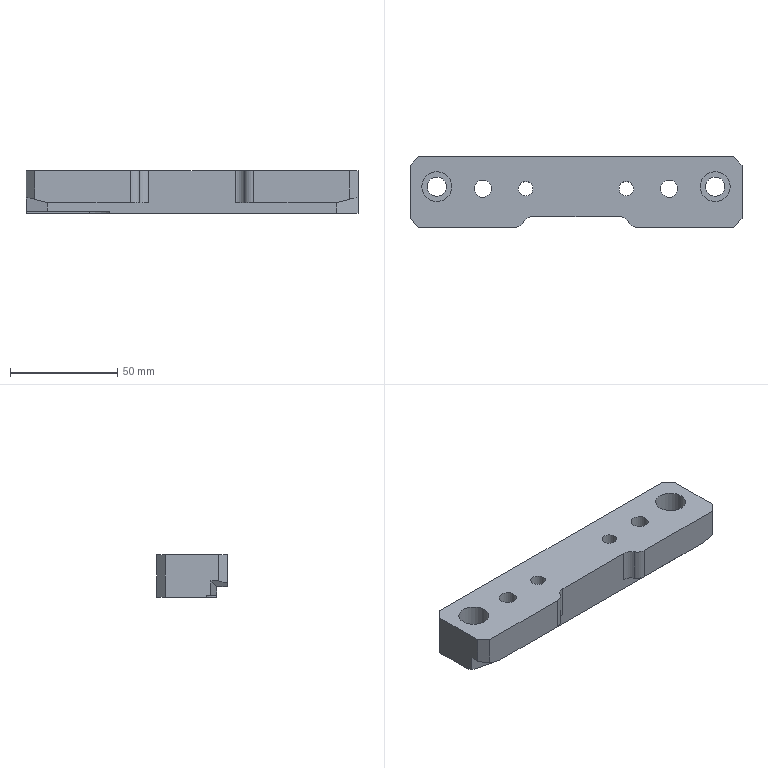Part | NX | features 20 2 | 1 solid | 35 faces | box 155 x 33 x 20 mm | volume 85943 mm3 | plane 22 | cylinder 13 | commonest cylinder face diameters 10 x4 6.8 x2 8.001 x2 9 x2 14 x2 24 x1
STEP:
#1=CARTESIAN_POINT('',(603.057,427.372,-2.5));
#2=VERTEX_POINT('',#1);
#3=CARTESIAN_POINT('',(612.711,422.5,-2.5));
#4=VERTEX_POINT('',#3);
#5=CARTESIAN_POINT('',(603.057,415.372,-2.5));
#6=DIRECTION('',(0.,0.,-1.));
#7=DIRECTION('',(1.,0.,0.));
#8=AXIS2_PLACEMENT_3D('',#5,#6,#7);
#9=CIRCLE('',#8,12.);
#10=EDGE_CURVE('',#2,#4,#9,.T.);
#11=ORIENTED_EDGE('',*,*,#10,.F.);
#12=CARTESIAN_POINT('',(603.057,427.372,-3.5));
#13=VERTEX_POINT('',#12);
#14=CARTESIAN_POINT('',(603.057,427.372,-33.5));
#15=DIRECTION('',(0.,0.,-1.));
#16=VECTOR('',#15,1000.);
#17=LINE('',#14,#16);
#18=EDGE_CURVE('',#2,#13,#17,.T.);
#19=ORIENTED_EDGE('',*,*,#18,.T.);
#20=CARTESIAN_POINT('',(612.711,422.5,-3.5));
#21=VERTEX_POINT('',#20);
#22=CARTESIAN_POINT('',(603.057,415.372,-3.5));
#23=DIRECTION('',(0.,0.,1.));
#24=DIRECTION('',(1.,0.,0.));
#25=AXIS2_PLACEMENT_3D('',#22,#23,#24);
#26=CIRCLE('',#25,12.);
#27=EDGE_CURVE('',#21,#13,#26,.T.);
#28=ORIENTED_EDGE('',*,*,#27,.F.);
#29=CARTESIAN_POINT('',(612.711,422.5,-33.5));
#30=DIRECTION('',(0.,0.,1.));
#31=VECTOR('',#30,1000.);
#32=LINE('',#29,#31);
#33=EDGE_CURVE('',#21,#4,#32,.T.);
#34=ORIENTED_EDGE('',*,*,#33,.T.);
#35=EDGE_LOOP('',(#11,#19,#28,#34));
#36=FACE_BOUND('',#35,.T.);
#37=CARTESIAN_POINT('',(603.057,415.372,-33.5));
#38=DIRECTION('',(0.,0.,1.));
#39=DIRECTION('',(-1.,0.,0.));
#40=AXIS2_PLACEMENT_3D('',#37,#38,#39);
#41=CYLINDRICAL_SURFACE('',#40,12.);
#42=ADVANCED_FACE('',(#36),#41,.F.);
#43=CARTESIAN_POINT('',(611.502,435.5,16.5));
#44=VERTEX_POINT('',#43);
#45=CARTESIAN_POINT('',(607.502,435.5,16.5));
#46=DIRECTION('',(0.,0.,1.));
#47=DIRECTION('',(1.,0.,0.));
#48=AXIS2_PLACEMENT_3D('',#45,#46,#47);
#49=CIRCLE('',#48,4.);
#50=EDGE_CURVE('',#44,#44,#49,.T.);
#51=ORIENTED_EDGE('',*,*,#50,.F.);
#52=EDGE_LOOP('',(#51));
#53=FACE_BOUND('',#52,.T.);
#54=CARTESIAN_POINT('',(698.502,435.5,16.5));
#55=VERTEX_POINT('',#54);
#56=CARTESIAN_POINT('',(694.502,435.5,16.5));
#57=DIRECTION('',(0.,0.,1.));
#58=DIRECTION('',(1.,0.,0.));
#59=AXIS2_PLACEMENT_3D('',#56,#57,#58);
#60=CIRCLE('',#59,4.);
#61=EDGE_CURVE('',#55,#55,#60,.T.);
#62=ORIENTED_EDGE('',*,*,#61,.F.);
#63=EDGE_LOOP('',(#62));
#64=FACE_BOUND('',#63,.T.);
#65=CARTESIAN_POINT('',(577.502,417.5,16.5));
#66=VERTEX_POINT('',#65);
#67=CARTESIAN_POINT('',(573.502,421.5,16.5));
#68=VERTEX_POINT('',#67);
#69=CARTESIAN_POINT('',(541.252,453.75,16.5));
#70=DIRECTION('',(-0.7071,0.7071,0.));
#71=VECTOR('',#70,1000.);
#72=LINE('',#69,#71);
#73=EDGE_CURVE('',#66,#68,#72,.T.);
#74=ORIENTED_EDGE('',*,*,#73,.F.);
#75=CARTESIAN_POINT('',(622.241,417.5,16.5));
#76=VERTEX_POINT('',#75);
#77=CARTESIAN_POINT('',(538.002,417.5,16.5));
#78=DIRECTION('',(-1.,0.,0.));
#79=VECTOR('',#78,1000.);
#80=LINE('',#77,#79);
#81=EDGE_CURVE('',#76,#66,#80,.T.);
#82=ORIENTED_EDGE('',*,*,#81,.F.);
#83=CARTESIAN_POINT('',(626.572,420.,16.5));
#84=VERTEX_POINT('',#83);
#85=CARTESIAN_POINT('',(622.241,422.5,16.5));
#86=DIRECTION('',(0.,0.,-1.));
#87=DIRECTION('',(1.,0.,0.));
#88=AXIS2_PLACEMENT_3D('',#85,#86,#87);
#89=CIRCLE('',#88,5.);
#90=EDGE_CURVE('',#84,#76,#89,.T.);
#91=ORIENTED_EDGE('',*,*,#90,.F.);
#92=CARTESIAN_POINT('',(630.902,422.5,16.5));
#93=VERTEX_POINT('',#92);
#94=CARTESIAN_POINT('',(630.902,417.5,16.5));
#95=DIRECTION('',(0.,0.,-1.));
#96=DIRECTION('',(1.,0.,0.));
#97=AXIS2_PLACEMENT_3D('',#94,#95,#96);
#98=CIRCLE('',#97,5.);
#99=EDGE_CURVE('',#84,#93,#98,.T.);
#100=ORIENTED_EDGE('',*,*,#99,.T.);
#101=CARTESIAN_POINT('',(671.102,422.5,16.5));
#102=VERTEX_POINT('',#101);
#103=CARTESIAN_POINT('',(538.002,422.5,16.5));
#104=DIRECTION('',(-1.,0.,0.));
#105=VECTOR('',#104,1000.);
#106=LINE('',#103,#105);
#107=EDGE_CURVE('',#102,#93,#106,.T.);
#108=ORIENTED_EDGE('',*,*,#107,.F.);
#109=CARTESIAN_POINT('',(675.432,420.,16.5));
#110=VERTEX_POINT('',#109);
#111=CARTESIAN_POINT('',(671.102,417.5,16.5));
#112=DIRECTION('',(0.,0.,1.));
#113=DIRECTION('',(1.,0.,0.));
#114=AXIS2_PLACEMENT_3D('',#111,#112,#113);
#115=CIRCLE('',#114,5.);
#116=EDGE_CURVE('',#110,#102,#115,.T.);
#117=ORIENTED_EDGE('',*,*,#116,.F.);
#118=CARTESIAN_POINT('',(679.762,417.5,16.5));
#119=VERTEX_POINT('',#118);
#120=CARTESIAN_POINT('',(679.762,422.5,16.5));
#121=DIRECTION('',(0.,0.,1.));
#122=DIRECTION('',(1.,0.,0.));
#123=AXIS2_PLACEMENT_3D('',#120,#121,#122);
#124=CIRCLE('',#123,5.);
#125=EDGE_CURVE('',#110,#119,#124,.T.);
#126=ORIENTED_EDGE('',*,*,#125,.T.);
#127=CARTESIAN_POINT('',(724.502,417.5,16.5));
#128=VERTEX_POINT('',#127);
#129=CARTESIAN_POINT('',(538.002,417.5,16.5));
#130=DIRECTION('',(1.,0.,0.));
#131=VECTOR('',#130,1000.);
#132=LINE('',#129,#131);
#133=EDGE_CURVE('',#119,#128,#132,.T.);
#134=ORIENTED_EDGE('',*,*,#133,.T.);
#135=CARTESIAN_POINT('',(728.502,421.5,16.5));
#136=VERTEX_POINT('',#135);
#137=CARTESIAN_POINT('',(724.502,417.5,16.5));
#138=DIRECTION('',(0.7071,0.7071,0.));
#139=VECTOR('',#138,1000.);
#140=LINE('',#137,#139);
#141=EDGE_CURVE('',#128,#136,#140,.T.);
#142=ORIENTED_EDGE('',*,*,#141,.T.);
#143=CARTESIAN_POINT('',(728.502,446.5,16.5));
#144=VERTEX_POINT('',#143);
#145=CARTESIAN_POINT('',(728.502,450.5,16.5));
#146=DIRECTION('',(0.,1.,0.));
#147=VECTOR('',#146,1000.);
#148=LINE('',#145,#147);
#149=EDGE_CURVE('',#136,#144,#148,.T.);
#150=ORIENTED_EDGE('',*,*,#149,.T.);
#151=CARTESIAN_POINT('',(724.502,450.5,16.5));
#152=VERTEX_POINT('',#151);
#153=CARTESIAN_POINT('',(728.502,446.5,16.5));
#154=DIRECTION('',(-0.7071,0.7071,0.));
#155=VECTOR('',#154,1000.);
#156=LINE('',#153,#155);
#157=EDGE_CURVE('',#144,#152,#156,.T.);
#158=ORIENTED_EDGE('',*,*,#157,.T.);
#159=CARTESIAN_POINT('',(577.502,450.5,16.5));
#160=VERTEX_POINT('',#159);
#161=CARTESIAN_POINT('',(458.002,450.5,16.5));
#162=DIRECTION('',(-1.,0.,0.));
#163=VECTOR('',#162,1000.);
#164=LINE('',#161,#163);
#165=EDGE_CURVE('',#152,#160,#164,.T.);
#166=ORIENTED_EDGE('',*,*,#165,.T.);
#167=CARTESIAN_POINT('',(573.502,446.5,16.5));
#168=VERTEX_POINT('',#167);
#169=CARTESIAN_POINT('',(559.252,432.25,16.5));
#170=DIRECTION('',(0.7071,0.7071,0.));
#171=VECTOR('',#170,1000.);
#172=LINE('',#169,#171);
#173=EDGE_CURVE('',#168,#160,#172,.T.);
#174=ORIENTED_EDGE('',*,*,#173,.F.);
#175=CARTESIAN_POINT('',(573.502,450.5,16.5));
#176=DIRECTION('',(0.,1.,0.));
#177=VECTOR('',#176,1000.);
#178=LINE('',#175,#177);
#179=EDGE_CURVE('',#68,#168,#178,.T.);
#180=ORIENTED_EDGE('',*,*,#179,.F.);
#181=EDGE_LOOP('',(#74,#82,#91,#100,#108,#117,#126,#134,#142,#150,#158,#166,#174,#180));
#182=FACE_BOUND('',#181,.T.);
#183=CARTESIAN_POINT('',(593.002,436.5,16.5));
#184=VERTEX_POINT('',#183);
#185=CARTESIAN_POINT('',(586.002,436.5,16.5));
#186=DIRECTION('',(0.,0.,1.));
#187=DIRECTION('',(1.,0.,0.));
#188=AXIS2_PLACEMENT_3D('',#185,#186,#187);
#189=CIRCLE('',#188,7.);
#190=EDGE_CURVE('',#184,#184,#189,.T.);
#191=ORIENTED_EDGE('',*,*,#190,.F.);
#192=EDGE_LOOP('',(#191));
#193=FACE_BOUND('',#192,.T.);
#194=CARTESIAN_POINT('',(723.002,436.5,16.5));
#195=VERTEX_POINT('',#194);
#196=CARTESIAN_POINT('',(716.002,436.5,16.5));
#197=DIRECTION('',(0.,0.,-1.));
#198=DIRECTION('',(1.,0.,0.));
#199=AXIS2_PLACEMENT_3D('',#196,#197,#198);
#200=CIRCLE('',#199,7.);
#201=EDGE_CURVE('',#195,#195,#200,.T.);
#202=ORIENTED_EDGE('',*,*,#201,.T.);
#203=EDGE_LOOP('',(#202));
#204=FACE_BOUND('',#203,.T.);
#205=CARTESIAN_POINT('',(677.902,435.5,16.5));
#206=VERTEX_POINT('',#205);
#207=CARTESIAN_POINT('',(674.502,435.5,16.5));
#208=DIRECTION('',(0.,0.,-1.));
#209=DIRECTION('',(1.,0.,0.));
#210=AXIS2_PLACEMENT_3D('',#207,#208,#209);
#211=CIRCLE('',#210,3.4);
#212=EDGE_CURVE('',#206,#206,#211,.T.);
#213=ORIENTED_EDGE('',*,*,#212,.T.);
#214=EDGE_LOOP('',(#213));
#215=FACE_BOUND('',#214,.T.);
#216=CARTESIAN_POINT('',(630.902,435.5,16.5));
#217=VERTEX_POINT('',#216);
#218=CARTESIAN_POINT('',(627.502,435.5,16.5));
#219=DIRECTION('',(0.,0.,1.));
#220=DIRECTION('',(1.,0.,0.));
#221=AXIS2_PLACEMENT_3D('',#218,#219,#220);
#222=CIRCLE('',#221,3.4);
#223=EDGE_CURVE('',#217,#217,#222,.T.);
#224=ORIENTED_EDGE('',*,*,#223,.F.);
#225=EDGE_LOOP('',(#224));
#226=FACE_BOUND('',#225,.T.);
#227=CARTESIAN_POINT('',(538.002,450.5,16.5));
#228=DIRECTION('',(0.,0.,1.));
#229=DIRECTION('',(-1.,0.,0.));
#230=AXIS2_PLACEMENT_3D('',#227,#228,#229);
#231=PLANE('',#230);
#232=ADVANCED_FACE('',(#53,#64,#182,#193,#204,#215,#226),#231,.T.);
#233=CARTESIAN_POINT('',(611.502,435.5,-3.5));
#234=VERTEX_POINT('',#233);
#235=CARTESIAN_POINT('',(607.502,435.5,-3.5));
#236=DIRECTION('',(0.,0.,-1.));
#237=DIRECTION('',(1.,0.,0.));
#238=AXIS2_PLACEMENT_3D('',#235,#236,#237);
#239=CIRCLE('',#238,4.);
#240=EDGE_CURVE('',#234,#234,#239,.T.);
#241=ORIENTED_EDGE('',*,*,#240,.F.);
#242=EDGE_LOOP('',(#241));
#243=FACE_BOUND('',#242,.T.);
#244=CARTESIAN_POINT('',(581.502,436.5,-3.5));
#245=VERTEX_POINT('',#244);
#246=CARTESIAN_POINT('',(586.002,436.5,-3.5));
#247=DIRECTION('',(0.,0.,-1.));
#248=DIRECTION('',(-1.,0.,0.));
#249=AXIS2_PLACEMENT_3D('',#246,#247,#248);
#250=CIRCLE('',#249,4.5);
#251=EDGE_CURVE('',#245,#245,#250,.T.);
#252=ORIENTED_EDGE('',*,*,#251,.F.);
#253=EDGE_LOOP('',(#252));
#254=FACE_BOUND('',#253,.T.);
#255=CARTESIAN_POINT('',(624.102,435.5,-3.5));
#256=VERTEX_POINT('',#255);
#257=CARTESIAN_POINT('',(627.502,435.5,-3.5));
#258=DIRECTION('',(0.,0.,1.));
#259=DIRECTION('',(-1.,0.,0.));
#260=AXIS2_PLACEMENT_3D('',#257,#258,#259);
#261=CIRCLE('',#260,3.4);
#262=EDGE_CURVE('',#256,#256,#261,.T.);
#263=ORIENTED_EDGE('',*,*,#262,.T.);
#264=EDGE_LOOP('',(#263));
#265=FACE_BOUND('',#264,.T.);
#266=CARTESIAN_POINT('',(698.502,435.5,-3.5));
#267=VERTEX_POINT('',#266);
#268=CARTESIAN_POINT('',(694.502,435.5,-3.5));
#269=DIRECTION('',(0.,0.,1.));
#270=DIRECTION('',(1.,0.,0.));
#271=AXIS2_PLACEMENT_3D('',#268,#269,#270);
#272=CIRCLE('',#271,4.);
#273=EDGE_CURVE('',#267,#267,#272,.T.);
#274=ORIENTED_EDGE('',*,*,#273,.T.);
#275=EDGE_LOOP('',(#274));
#276=FACE_BOUND('',#275,.T.);
#277=CARTESIAN_POINT('',(720.502,436.5,-3.5));
#278=VERTEX_POINT('',#277);
#279=CARTESIAN_POINT('',(716.002,436.5,-3.5));
#280=DIRECTION('',(0.,0.,1.));
#281=DIRECTION('',(1.,0.,0.));
#282=AXIS2_PLACEMENT_3D('',#279,#280,#281);
#283=CIRCLE('',#282,4.5);
#284=EDGE_CURVE('',#278,#278,#283,.T.);
#285=ORIENTED_EDGE('',*,*,#284,.T.);
#286=EDGE_LOOP('',(#285));
#287=FACE_BOUND('',#286,.T.);
#288=CARTESIAN_POINT('',(677.902,435.5,-3.5));
#289=VERTEX_POINT('',#288);
#290=CARTESIAN_POINT('',(674.502,435.5,-3.5));
#291=DIRECTION('',(0.,0.,-1.));
#292=DIRECTION('',(1.,0.,0.));
#293=AXIS2_PLACEMENT_3D('',#290,#291,#292);
#294=CIRCLE('',#293,3.4);
#295=EDGE_CURVE('',#289,#289,#294,.T.);
#296=ORIENTED_EDGE('',*,*,#295,.F.);
#297=EDGE_LOOP('',(#296));
#298=FACE_BOUND('',#297,.T.);
#299=CARTESIAN_POINT('',(728.502,425.18,-3.5));
#300=VERTEX_POINT('',#299);
#301=CARTESIAN_POINT('',(728.502,446.5,-3.5));
#302=VERTEX_POINT('',#301);
#303=CARTESIAN_POINT('',(728.502,450.5,-3.5));
#304=DIRECTION('',(0.,1.,0.));
#305=VECTOR('',#304,1000.);
#306=LINE('',#303,#305);
#307=EDGE_CURVE('',#300,#302,#306,.T.);
#308=ORIENTED_EDGE('',*,*,#307,.F.);
#309=CARTESIAN_POINT('',(718.5,422.5,-3.5));
#310=VERTEX_POINT('',#309);
#311=CARTESIAN_POINT('',(728.502,425.18,-3.5));
#312=DIRECTION('',(0.9659,0.2588,0.));
#313=VECTOR('',#312,1000.);
#314=LINE('',#311,#313);
#315=EDGE_CURVE('',#310,#300,#314,.T.);
#316=ORIENTED_EDGE('',*,*,#315,.F.);
#317=CARTESIAN_POINT('',(528.,422.5,-3.5));
#318=DIRECTION('',(1.,0.,0.));
#319=VECTOR('',#318,1000.);
#320=LINE('',#317,#319);
#321=EDGE_CURVE('',#21,#310,#320,.T.);
#322=ORIENTED_EDGE('',*,*,#321,.F.);
#323=ORIENTED_EDGE('',*,*,#27,.T.);
#324=CARTESIAN_POINT('',(573.502,427.372,-3.5));
#325=VERTEX_POINT('',#324);
#326=CARTESIAN_POINT('',(603.057,427.372,-3.5));
#327=DIRECTION('',(1.,0.,0.));
#328=VECTOR('',#327,1000.);
#329=LINE('',#326,#328);
#330=EDGE_CURVE('',#325,#13,#329,.T.);
#331=ORIENTED_EDGE('',*,*,#330,.F.);
#332=CARTESIAN_POINT('',(573.502,446.5,-3.5));
#333=VERTEX_POINT('',#332);
#334=CARTESIAN_POINT('',(573.502,450.5,-3.5));
#335=DIRECTION('',(0.,1.,0.));
#336=VECTOR('',#335,1000.);
#337=LINE('',#334,#336);
#338=EDGE_CURVE('',#325,#333,#337,.T.);
#339=ORIENTED_EDGE('',*,*,#338,.T.);
#340=CARTESIAN_POINT('',(577.502,450.5,-3.5));
#341=VERTEX_POINT('',#340);
#342=CARTESIAN_POINT('',(573.502,446.5,-3.5));
#343=DIRECTION('',(-0.7071,-0.7071,0.));
#344=VECTOR('',#343,1000.);
#345=LINE('',#342,#344);
#346=EDGE_CURVE('',#341,#333,#345,.T.);
#347=ORIENTED_EDGE('',*,*,#346,.F.);
#348=CARTESIAN_POINT('',(724.502,450.5,-3.5));
#349=VERTEX_POINT('',#348);
#350=CARTESIAN_POINT('',(458.002,450.5,-3.5));
#351=DIRECTION('',(-1.,0.,0.));
#352=VECTOR('',#351,1000.);
#353=LINE('',#350,#352);
#354=EDGE_CURVE('',#349,#341,#353,.T.);
#355=ORIENTED_EDGE('',*,*,#354,.F.);
#356=CARTESIAN_POINT('',(728.502,446.5,-3.5));
#357=DIRECTION('',(0.7071,-0.7071,0.));
#358=VECTOR('',#357,1000.);
#359=LINE('',#356,#358);
#360=EDGE_CURVE('',#349,#302,#359,.T.);
#361=ORIENTED_EDGE('',*,*,#360,.T.);
#362=EDGE_LOOP('',(#308,#316,#322,#323,#331,#339,#347,#355,#361));
#363=FACE_BOUND('',#362,.T.);
#364=CARTESIAN_POINT('',(538.002,450.5,-3.5));
#365=DIRECTION('',(0.,0.,1.));
#366=DIRECTION('',(-1.,0.,0.));
#367=AXIS2_PLACEMENT_3D('',#364,#365,#366);
#368=PLANE('',#367);
#369=ADVANCED_FACE('',(#243,#254,#265,#276,#287,#298,#363),#368,.F.);
#370=CARTESIAN_POINT('',(728.502,425.18,4.179));
#371=VERTEX_POINT('',#370);
#372=CARTESIAN_POINT('',(728.502,425.18,3.5));
#373=DIRECTION('',(0.,0.,1.));
#374=VECTOR('',#373,1000.);
#375=LINE('',#372,#374);
#376=EDGE_CURVE('',#300,#371,#375,.T.);
#377=ORIENTED_EDGE('',*,*,#376,.F.);
#378=ORIENTED_EDGE('',*,*,#307,.T.);
#379=CARTESIAN_POINT('',(728.502,446.5,11.5));
#380=DIRECTION('',(0.,0.,1.));
#381=VECTOR('',#380,1000.);
#382=LINE('',#379,#381);
#383=EDGE_CURVE('',#302,#144,#382,.T.);
#384=ORIENTED_EDGE('',*,*,#383,.T.);
#385=ORIENTED_EDGE('',*,*,#149,.F.);
#386=CARTESIAN_POINT('',(728.502,421.5,4.179));
#387=VERTEX_POINT('',#386);
#388=CARTESIAN_POINT('',(728.502,421.5,11.5));
#389=DIRECTION('',(0.,0.,-1.));
#390=VECTOR('',#389,1000.);
#391=LINE('',#388,#390);
#392=EDGE_CURVE('',#136,#387,#391,.T.);
#393=ORIENTED_EDGE('',*,*,#392,.T.);
#394=CARTESIAN_POINT('',(728.502,417.5,4.179));
#395=DIRECTION('',(0.,1.,0.));
#396=VECTOR('',#395,1000.);
#397=LINE('',#394,#396);
#398=EDGE_CURVE('',#387,#371,#397,.T.);
#399=ORIENTED_EDGE('',*,*,#398,.T.);
#400=EDGE_LOOP('',(#377,#378,#384,#385,#393,#399));
#401=FACE_BOUND('',#400,.T.);
#402=CARTESIAN_POINT('',(728.502,450.5,11.5));
#403=DIRECTION('',(-1.,0.,0.));
#404=DIRECTION('',(0.,0.,-1.));
#405=AXIS2_PLACEMENT_3D('',#402,#403,#404);
#406=PLANE('',#405);
#407=ADVANCED_FACE('',(#401),#406,.F.);
#408=ORIENTED_EDGE('',*,*,#338,.F.);
#409=CARTESIAN_POINT('',(573.502,427.372,-2.5));
#410=VERTEX_POINT('',#409);
#411=CARTESIAN_POINT('',(573.502,427.372,-33.5));
#412=DIRECTION('',(0.,0.,-1.));
#413=VECTOR('',#412,1000.);
#414=LINE('',#411,#413);
#415=EDGE_CURVE('',#410,#325,#414,.T.);
#416=ORIENTED_EDGE('',*,*,#415,.F.);
#417=CARTESIAN_POINT('',(573.502,425.18,-2.5));
#418=VERTEX_POINT('',#417);
#419=CARTESIAN_POINT('',(573.502,450.5,-2.5));
#420=DIRECTION('',(0.,1.,0.));
#421=VECTOR('',#420,1000.);
#422=LINE('',#419,#421);
#423=EDGE_CURVE('',#418,#410,#422,.T.);
#424=ORIENTED_EDGE('',*,*,#423,.F.);
#425=CARTESIAN_POINT('',(573.502,425.18,4.179));
#426=VERTEX_POINT('',#425);
#427=CARTESIAN_POINT('',(573.502,425.18,3.5));
#428=DIRECTION('',(0.,0.,1.));
#429=VECTOR('',#428,1000.);
#430=LINE('',#427,#429);
#431=EDGE_CURVE('',#418,#426,#430,.T.);
#432=ORIENTED_EDGE('',*,*,#431,.T.);
#433=CARTESIAN_POINT('',(573.502,421.5,4.179));
#434=VERTEX_POINT('',#433);
#435=CARTESIAN_POINT('',(573.502,417.5,4.179));
#436=DIRECTION('',(0.,1.,0.));
#437=VECTOR('',#436,1000.);
#438=LINE('',#435,#437);
#439=EDGE_CURVE('',#434,#426,#438,.T.);
#440=ORIENTED_EDGE('',*,*,#439,.F.);
#441=CARTESIAN_POINT('',(573.502,421.5,11.5));
#442=DIRECTION('',(0.,0.,-1.));
#443=VECTOR('',#442,1000.);
#444=LINE('',#441,#443);
#445=EDGE_CURVE('',#68,#434,#444,.T.);
#446=ORIENTED_EDGE('',*,*,#445,.F.);
#447=ORIENTED_EDGE('',*,*,#179,.T.);
#448=CARTESIAN_POINT('',(573.502,446.5,11.5));
#449=DIRECTION('',(0.,0.,1.));
#450=VECTOR('',#449,1000.);
#451=LINE('',#448,#450);
#452=EDGE_CURVE('',#333,#168,#451,.T.);
#453=ORIENTED_EDGE('',*,*,#452,.F.);
#454=EDGE_LOOP('',(#408,#416,#424,#432,#440,#446,#447,#453));
#455=FACE_BOUND('',#454,.T.);
#456=CARTESIAN_POINT('',(573.502,450.5,11.5));
#457=DIRECTION('',(1.,0.,0.));
#458=DIRECTION('',(0.,0.,-1.));
#459=AXIS2_PLACEMENT_3D('',#456,#457,#458);
#460=PLANE('',#459);
#461=ADVANCED_FACE('',(#455),#460,.F.);
#462=ORIENTED_EDGE('',*,*,#354,.T.);
#463=CARTESIAN_POINT('',(577.502,450.5,11.5));
#464=DIRECTION('',(0.,0.,-1.));
#465=VECTOR('',#464,1000.);
#466=LINE('',#463,#465);
#467=EDGE_CURVE('',#160,#341,#466,.T.);
#468=ORIENTED_EDGE('',*,*,#467,.F.);
#469=ORIENTED_EDGE('',*,*,#165,.F.);
#470=CARTESIAN_POINT('',(724.502,450.5,11.5));
#471=DIRECTION('',(0.,0.,-1.));
#472=VECTOR('',#471,1000.);
#473=LINE('',#470,#472);
#474=EDGE_CURVE('',#152,#349,#473,.T.);
#475=ORIENTED_EDGE('',*,*,#474,.T.);
#476=EDGE_LOOP('',(#462,#468,#469,#475));
#477=FACE_BOUND('',#476,.T.);
#478=CARTESIAN_POINT('',(458.002,450.5,11.5));
#479=DIRECTION('',(0.,-1.,0.));
#480=DIRECTION('',(0.,0.,-1.));
#481=AXIS2_PLACEMENT_3D('',#478,#479,#480);
#482=PLANE('',#481);
#483=ADVANCED_FACE('',(#477),#482,.F.);
#484=ORIENTED_EDGE('',*,*,#273,.F.);
#485=EDGE_LOOP('',(#484));
#486=FACE_BOUND('',#485,.T.);
#487=ORIENTED_EDGE('',*,*,#61,.T.);
#488=EDGE_LOOP('',(#487));
#489=FACE_BOUND('',#488,.T.);
#490=CARTESIAN_POINT('',(694.502,435.5,42.5));
#491=DIRECTION('',(0.,0.,-1.));
#492=DIRECTION('',(1.,0.,0.));
#493=AXIS2_PLACEMENT_3D('',#490,#491,#492);
#494=CYLINDRICAL_SURFACE('',#493,4.);
#495=ADVANCED_FACE('',(#486,#489),#494,.F.);
#496=ORIENTED_EDGE('',*,*,#201,.F.);
#497=EDGE_LOOP('',(#496));
#498=FACE_BOUND('',#497,.T.);
#499=CARTESIAN_POINT('',(723.002,436.5,6.5));
#500=VERTEX_POINT('',#499);
#501=CARTESIAN_POINT('',(716.002,436.5,6.5));
#502=DIRECTION('',(0.,0.,1.));
#503=DIRECTION('',(1.,0.,0.));
#504=AXIS2_PLACEMENT_3D('',#501,#502,#503);
#505=CIRCLE('',#504,7.);
#506=EDGE_CURVE('',#500,#500,#505,.T.);
#507=ORIENTED_EDGE('',*,*,#506,.F.);
#508=EDGE_LOOP('',(#507));
#509=FACE_BOUND('',#508,.T.);
#510=CARTESIAN_POINT('',(716.002,436.5,11.5));
#511=DIRECTION('',(0.,0.,-1.));
#512=DIRECTION('',(-1.,0.,0.));
#513=AXIS2_PLACEMENT_3D('',#510,#511,#512);
#514=CYLINDRICAL_SURFACE('',#513,7.);
#515=ADVANCED_FACE('',(#498,#509),#514,.F.);
#516=ORIENTED_EDGE('',*,*,#383,.F.);
#517=ORIENTED_EDGE('',*,*,#360,.F.);
#518=ORIENTED_EDGE('',*,*,#474,.F.);
#519=ORIENTED_EDGE('',*,*,#157,.F.);
#520=EDGE_LOOP('',(#516,#517,#518,#519));
#521=FACE_BOUND('',#520,.T.);
#522=CARTESIAN_POINT('',(728.502,446.5,11.5));
#523=DIRECTION('',(-0.7071,-0.7071,0.));
#524=DIRECTION('',(0.,0.,-1.));
#525=AXIS2_PLACEMENT_3D('',#522,#523,#524);
#526=PLANE('',#525);
#527=ADVANCED_FACE('',(#521),#526,.F.);
#528=CARTESIAN_POINT('',(720.502,436.5,6.5));
#529=VERTEX_POINT('',#528);
#530=CARTESIAN_POINT('',(716.002,436.5,6.5));
#531=DIRECTION('',(0.,0.,1.));
#532=DIRECTION('',(1.,0.,0.));
#533=AXIS2_PLACEMENT_3D('',#530,#531,#532);
#534=CIRCLE('',#533,4.5);
#535=EDGE_CURVE('',#529,#529,#534,.T.);
#536=ORIENTED_EDGE('',*,*,#535,.F.);
#537=EDGE_LOOP('',(#536));
#538=FACE_BOUND('',#537,.T.);
#539=ORIENTED_EDGE('',*,*,#506,.T.);
#540=EDGE_LOOP('',(#539));
#541=FACE_BOUND('',#540,.T.);
#542=CARTESIAN_POINT('',(855.502,302.3,6.5));
#543=DIRECTION('',(0.,0.,1.));
#544=DIRECTION('',(0.,1.,0.));
#545=AXIS2_PLACEMENT_3D('',#542,#543,#544);
#546=PLANE('',#545);
#547=ADVANCED_FACE('',(#538,#541),#546,.T.);
#548=ORIENTED_EDGE('',*,*,#535,.T.);
#549=EDGE_LOOP('',(#548));
#550=FACE_BOUND('',#549,.T.);
#551=ORIENTED_EDGE('',*,*,#284,.F.);
#552=EDGE_LOOP('',(#551));
#553=FACE_BOUND('',#552,.T.);
#554=CARTESIAN_POINT('',(716.002,436.5,-18.5));
#555=DIRECTION('',(0.,0.,-1.));
#556=DIRECTION('',(-1.,0.,0.));
#557=AXIS2_PLACEMENT_3D('',#554,#555,#556);
#558=CYLINDRICAL_SURFACE('',#557,4.5);
#559=ADVANCED_FACE('',(#550,#553),#558,.F.);
#560=ORIENTED_EDGE('',*,*,#212,.F.);
#561=EDGE_LOOP('',(#560));
#562=FACE_BOUND('',#561,.T.);
#563=ORIENTED_EDGE('',*,*,#295,.T.);
#564=EDGE_LOOP('',(#563));
#565=FACE_BOUND('',#564,.T.);
#566=CARTESIAN_POINT('',(674.502,435.5,-671.5));
#567=DIRECTION('',(0.,0.,1.));
#568=DIRECTION('',(1.,0.,0.));
#569=AXIS2_PLACEMENT_3D('',#566,#567,#568);
#570=CYLINDRICAL_SURFACE('',#569,3.4);
#571=ADVANCED_FACE('',(#562,#565),#570,.F.);
#572=ORIENTED_EDGE('',*,*,#240,.T.);
#573=EDGE_LOOP('',(#572));
#574=FACE_BOUND('',#573,.T.);
#575=ORIENTED_EDGE('',*,*,#50,.T.);
#576=EDGE_LOOP('',(#575));
#577=FACE_BOUND('',#576,.T.);
#578=CARTESIAN_POINT('',(607.502,435.5,42.5));
#579=DIRECTION('',(0.,0.,-1.));
#580=DIRECTION('',(-1.,0.,0.));
#581=AXIS2_PLACEMENT_3D('',#578,#579,#580);
#582=CYLINDRICAL_SURFACE('',#581,4.);
#583=ADVANCED_FACE('',(#574,#577),#582,.F.);
#584=ORIENTED_EDGE('',*,*,#190,.T.);
#585=EDGE_LOOP('',(#584));
#586=FACE_BOUND('',#585,.T.);
#587=CARTESIAN_POINT('',(593.002,436.5,6.5));
#588=VERTEX_POINT('',#587);
#589=CARTESIAN_POINT('',(586.002,436.5,6.5));
#590=DIRECTION('',(0.,0.,-1.));
#591=DIRECTION('',(1.,0.,0.));
#592=AXIS2_PLACEMENT_3D('',#589,#590,#591);
#593=CIRCLE('',#592,7.);
#594=EDGE_CURVE('',#588,#588,#593,.T.);
#595=ORIENTED_EDGE('',*,*,#594,.T.);
#596=EDGE_LOOP('',(#595));
#597=FACE_BOUND('',#596,.T.);
#598=CARTESIAN_POINT('',(586.002,436.5,11.5));
#599=DIRECTION('',(0.,0.,-1.));
#600=DIRECTION('',(1.,0.,0.));
#601=AXIS2_PLACEMENT_3D('',#598,#599,#600);
#602=CYLINDRICAL_SURFACE('',#601,7.);
#603=ADVANCED_FACE('',(#586,#597),#602,.F.);
#604=ORIENTED_EDGE('',*,*,#452,.T.);
#605=ORIENTED_EDGE('',*,*,#173,.T.);
#606=ORIENTED_EDGE('',*,*,#467,.T.);
#607=ORIENTED_EDGE('',*,*,#346,.T.);
#608=EDGE_LOOP('',(#604,#605,#606,#607));
#609=FACE_BOUND('',#608,.T.);
#610=CARTESIAN_POINT('',(573.502,446.5,11.5));
#611=DIRECTION('',(0.7071,-0.7071,0.));
#612=DIRECTION('',(0.,0.,-1.));
#613=AXIS2_PLACEMENT_3D('',#610,#611,#612);
#614=PLANE('',#613);
#615=ADVANCED_FACE('',(#609),#614,.F.);
#616=CARTESIAN_POINT('',(590.502,436.5,6.5));
#617=VERTEX_POINT('',#616);
#618=CARTESIAN_POINT('',(586.002,436.5,6.5));
#619=DIRECTION('',(0.,0.,-1.));
#620=DIRECTION('',(1.,0.,0.));
#621=AXIS2_PLACEMENT_3D('',#618,#619,#620);
#622=CIRCLE('',#621,4.5);
#623=EDGE_CURVE('',#617,#617,#622,.T.);
#624=ORIENTED_EDGE('',*,*,#623,.T.);
#625=EDGE_LOOP('',(#624));
#626=FACE_BOUND('',#625,.T.);
#627=ORIENTED_EDGE('',*,*,#594,.F.);
#628=EDGE_LOOP('',(#627));
#629=FACE_BOUND('',#628,.T.);
#630=CARTESIAN_POINT('',(446.502,302.3,6.5));
#631=DIRECTION('',(0.,0.,1.));
#632=DIRECTION('',(0.,1.,0.));
#633=AXIS2_PLACEMENT_3D('',#630,#631,#632);
#634=PLANE('',#633);
#635=ADVANCED_FACE('',(#626,#629),#634,.T.);
#636=ORIENTED_EDGE('',*,*,#623,.F.);
#637=EDGE_LOOP('',(#636));
#638=FACE_BOUND('',#637,.T.);
#639=ORIENTED_EDGE('',*,*,#251,.T.);
#640=EDGE_LOOP('',(#639));
#641=FACE_BOUND('',#640,.T.);
#642=CARTESIAN_POINT('',(586.002,436.5,-18.5));
#643=DIRECTION('',(0.,0.,-1.));
#644=DIRECTION('',(1.,0.,0.));
#645=AXIS2_PLACEMENT_3D('',#642,#643,#644);
#646=CYLINDRICAL_SURFACE('',#645,4.5);
#647=ADVANCED_FACE('',(#638,#641),#646,.F.);
#648=ORIENTED_EDGE('',*,*,#223,.T.);
#649=EDGE_LOOP('',(#648));
#650=FACE_BOUND('',#649,.T.);
#651=ORIENTED_EDGE('',*,*,#262,.F.);
#652=EDGE_LOOP('',(#651));
#653=FACE_BOUND('',#652,.T.);
#654=CARTESIAN_POINT('',(627.502,435.5,-671.5));
#655=DIRECTION('',(0.,0.,1.));
#656=DIRECTION('',(-1.,0.,0.));
#657=AXIS2_PLACEMENT_3D('',#654,#655,#656);
#658=CYLINDRICAL_SURFACE('',#657,3.4);
#659=ADVANCED_FACE('',(#650,#653),#658,.F.);
#660=CARTESIAN_POINT('',(718.502,417.5,1.5));
#661=VERTEX_POINT('',#660);
#662=CARTESIAN_POINT('',(679.762,417.5,1.5));
#663=VERTEX_POINT('',#662);
#664=CARTESIAN_POINT('',(538.002,417.5,1.5));
#665=DIRECTION('',(-1.,0.,0.));
#666=VECTOR('',#665,1000.);
#667=LINE('',#664,#666);
#668=EDGE_CURVE('',#661,#663,#667,.T.);
#669=ORIENTED_EDGE('',*,*,#668,.T.);
#670=CARTESIAN_POINT('',(675.432,420.,1.5));
#671=VERTEX_POINT('',#670);
#672=CARTESIAN_POINT('',(679.762,422.5,1.5));
#673=DIRECTION('',(0.,0.,-1.));
#674=DIRECTION('',(-1.,0.,0.));
#675=AXIS2_PLACEMENT_3D('',#672,#673,#674);
#676=CIRCLE('',#675,5.);
#677=EDGE_CURVE('',#663,#671,#676,.T.);
#678=ORIENTED_EDGE('',*,*,#677,.T.);
#679=CARTESIAN_POINT('',(671.102,422.5,1.5));
#680=VERTEX_POINT('',#679);
#681=CARTESIAN_POINT('',(671.102,417.5,1.5));
#682=DIRECTION('',(0.,0.,-1.));
#683=DIRECTION('',(-1.,0.,0.));
#684=AXIS2_PLACEMENT_3D('',#681,#682,#683);
#685=CIRCLE('',#684,5.);
#686=EDGE_CURVE('',#680,#671,#685,.T.);
#687=ORIENTED_EDGE('',*,*,#686,.F.);
#688=CARTESIAN_POINT('',(718.5,422.5,1.5));
#689=VERTEX_POINT('',#688);
#690=CARTESIAN_POINT('',(528.,422.5,1.5));
#691=DIRECTION('',(-1.,0.,0.));
#692=VECTOR('',#691,1000.);
#693=LINE('',#690,#692);
#694=EDGE_CURVE('',#689,#680,#693,.T.);
#695=ORIENTED_EDGE('',*,*,#694,.F.);
#696=CARTESIAN_POINT('',(718.502,422.5,1.5));
#697=VERTEX_POINT('',#696);
#698=CARTESIAN_POINT('',(728.502,425.18,1.5));
#699=DIRECTION('',(-0.9659,-0.2588,0.));
#700=VECTOR('',#699,1000.);
#701=LINE('',#698,#700);
#702=EDGE_CURVE('',#697,#689,#701,.T.);
#703=ORIENTED_EDGE('',*,*,#702,.F.);
#704=CARTESIAN_POINT('',(718.502,425.18,1.5));
#705=DIRECTION('',(0.,-1.,0.));
#706=VECTOR('',#705,1000.);
#707=LINE('',#704,#706);
#708=EDGE_CURVE('',#697,#661,#707,.T.);
#709=ORIENTED_EDGE('',*,*,#708,.T.);
#710=EDGE_LOOP('',(#669,#678,#687,#695,#703,#709));
#711=FACE_BOUND('',#710,.T.);
#712=CARTESIAN_POINT('',(560.272,396.891,1.5));
#713=DIRECTION('',(0.,0.,-1.));
#714=DIRECTION('',(1.,0.,0.));
#715=AXIS2_PLACEMENT_3D('',#712,#713,#714);
#716=PLANE('',#715);
#717=ADVANCED_FACE('',(#711),#716,.T.);
#718=CARTESIAN_POINT('',(583.502,417.5,1.5));
#719=VERTEX_POINT('',#718);
#720=CARTESIAN_POINT('',(622.241,417.5,1.5));
#721=VERTEX_POINT('',#720);
#722=CARTESIAN_POINT('',(764.002,417.5,1.5));
#723=DIRECTION('',(1.,0.,0.));
#724=VECTOR('',#723,1000.);
#725=LINE('',#722,#724);
#726=EDGE_CURVE('',#719,#721,#725,.T.);
#727=ORIENTED_EDGE('',*,*,#726,.F.);
#728=CARTESIAN_POINT('',(583.502,422.5,1.5));
#729=VERTEX_POINT('',#728);
#730=CARTESIAN_POINT('',(583.502,425.18,1.5));
#731=DIRECTION('',(0.,-1.,0.));
#732=VECTOR('',#731,1000.);
#733=LINE('',#730,#732);
#734=EDGE_CURVE('',#729,#719,#733,.T.);
#735=ORIENTED_EDGE('',*,*,#734,.F.);
#736=CARTESIAN_POINT('',(583.503,422.5,1.5));
#737=VERTEX_POINT('',#736);
#738=CARTESIAN_POINT('',(573.502,425.18,1.5));
#739=DIRECTION('',(0.9659,-0.2588,0.));
#740=VECTOR('',#739,1000.);
#741=LINE('',#738,#740);
#742=EDGE_CURVE('',#729,#737,#741,.T.);
#743=ORIENTED_EDGE('',*,*,#742,.T.);
#744=CARTESIAN_POINT('',(630.902,422.5,1.5));
#745=VERTEX_POINT('',#744);
#746=CARTESIAN_POINT('',(774.003,422.5,1.5));
#747=DIRECTION('',(1.,0.,0.));
#748=VECTOR('',#747,1000.);
#749=LINE('',#746,#748);
#750=EDGE_CURVE('',#737,#745,#749,.T.);
#751=ORIENTED_EDGE('',*,*,#750,.T.);
#752=CARTESIAN_POINT('',(626.572,420.,1.5));
#753=VERTEX_POINT('',#752);
#754=CARTESIAN_POINT('',(630.902,417.5,1.5));
#755=DIRECTION('',(0.,0.,1.));
#756=DIRECTION('',(1.,0.,0.));
#757=AXIS2_PLACEMENT_3D('',#754,#755,#756);
#758=CIRCLE('',#757,5.);
#759=EDGE_CURVE('',#745,#753,#758,.T.);
#760=ORIENTED_EDGE('',*,*,#759,.T.);
#761=CARTESIAN_POINT('',(622.241,422.5,1.5));
#762=DIRECTION('',(0.,0.,1.));
#763=DIRECTION('',(1.,0.,0.));
#764=AXIS2_PLACEMENT_3D('',#761,#762,#763);
#765=CIRCLE('',#764,5.);
#766=EDGE_CURVE('',#721,#753,#765,.T.);
#767=ORIENTED_EDGE('',*,*,#766,.F.);
#768=EDGE_LOOP('',(#727,#735,#743,#751,#760,#767));
#769=FACE_BOUND('',#768,.T.);
#770=CARTESIAN_POINT('',(741.731,396.891,1.5));
#771=DIRECTION('',(0.,0.,-1.));
#772=DIRECTION('',(-1.,0.,0.));
#773=AXIS2_PLACEMENT_3D('',#770,#771,#772);
#774=PLANE('',#773);
#775=ADVANCED_FACE('',(#769),#774,.T.);
#776=ORIENTED_EDGE('',*,*,#133,.F.);
#777=CARTESIAN_POINT('',(679.762,417.5,11.5));
#778=DIRECTION('',(0.,0.,-1.));
#779=VECTOR('',#778,1000.);
#780=LINE('',#777,#779);
#781=EDGE_CURVE('',#119,#663,#780,.T.);
#782=ORIENTED_EDGE('',*,*,#781,.T.);
#783=ORIENTED_EDGE('',*,*,#668,.F.);
#784=CARTESIAN_POINT('',(724.502,417.5,3.108));
#785=VERTEX_POINT('',#784);
#786=CARTESIAN_POINT('',(718.502,417.5,1.5));
#787=DIRECTION('',(0.9659,0.,0.2588));
#788=VECTOR('',#787,1000.);
#789=LINE('',#786,#788);
#790=EDGE_CURVE('',#661,#785,#789,.T.);
#791=ORIENTED_EDGE('',*,*,#790,.T.);
#792=CARTESIAN_POINT('',(724.502,417.5,11.5));
#793=DIRECTION('',(0.,0.,1.));
#794=VECTOR('',#793,1000.);
#795=LINE('',#792,#794);
#796=EDGE_CURVE('',#785,#128,#795,.T.);
#797=ORIENTED_EDGE('',*,*,#796,.T.);
#798=EDGE_LOOP('',(#776,#782,#783,#791,#797));
#799=FACE_BOUND('',#798,.T.);
#800=CARTESIAN_POINT('',(538.002,417.5,11.5));
#801=DIRECTION('',(0.,1.,0.));
#802=DIRECTION('',(0.,0.,1.));
#803=AXIS2_PLACEMENT_3D('',#800,#801,#802);
#804=PLANE('',#803);
#805=ADVANCED_FACE('',(#799),#804,.F.);
#806=ORIENTED_EDGE('',*,*,#677,.F.);
#807=ORIENTED_EDGE('',*,*,#781,.F.);
#808=ORIENTED_EDGE('',*,*,#125,.F.);
#809=CARTESIAN_POINT('',(675.432,420.,-10.));
#810=DIRECTION('',(0.,0.,1.));
#811=VECTOR('',#810,1000.);
#812=LINE('',#809,#811);
#813=EDGE_CURVE('',#671,#110,#812,.T.);
#814=ORIENTED_EDGE('',*,*,#813,.F.);
#815=EDGE_LOOP('',(#806,#807,#808,#814));
#816=FACE_BOUND('',#815,.T.);
#817=CARTESIAN_POINT('',(679.762,422.5,-10.));
#818=DIRECTION('',(0.,0.,1.));
#819=DIRECTION('',(-1.,0.,0.));
#820=AXIS2_PLACEMENT_3D('',#817,#818,#819);
#821=CYLINDRICAL_SURFACE('',#820,5.);
#822=ADVANCED_FACE('',(#816),#821,.T.);
#823=ORIENTED_EDGE('',*,*,#686,.T.);
#824=ORIENTED_EDGE('',*,*,#813,.T.);
#825=ORIENTED_EDGE('',*,*,#116,.T.);
#826=CARTESIAN_POINT('',(671.102,422.5,3.5));
#827=DIRECTION('',(0.,0.,-1.));
#828=VECTOR('',#827,1000.);
#829=LINE('',#826,#828);
#830=EDGE_CURVE('',#102,#680,#829,.T.);
#831=ORIENTED_EDGE('',*,*,#830,.T.);
#832=EDGE_LOOP('',(#823,#824,#825,#831));
#833=FACE_BOUND('',#832,.T.);
#834=CARTESIAN_POINT('',(671.102,417.5,-10.));
#835=DIRECTION('',(0.,0.,1.));
#836=DIRECTION('',(-1.,0.,0.));
#837=AXIS2_PLACEMENT_3D('',#834,#835,#836);
#838=CYLINDRICAL_SURFACE('',#837,5.);
#839=ADVANCED_FACE('',(#833),#838,.F.);
#840=ORIENTED_EDGE('',*,*,#759,.F.);
#841=CARTESIAN_POINT('',(630.902,422.5,3.5));
#842=DIRECTION('',(0.,0.,-1.));
#843=VECTOR('',#842,1000.);
#844=LINE('',#841,#843);
#845=EDGE_CURVE('',#93,#745,#844,.T.);
#846=ORIENTED_EDGE('',*,*,#845,.F.);
#847=ORIENTED_EDGE('',*,*,#99,.F.);
#848=CARTESIAN_POINT('',(626.572,420.,-10.));
#849=DIRECTION('',(0.,0.,1.));
#850=VECTOR('',#849,1000.);
#851=LINE('',#848,#850);
#852=EDGE_CURVE('',#753,#84,#851,.T.);
#853=ORIENTED_EDGE('',*,*,#852,.F.);
#854=EDGE_LOOP('',(#840,#846,#847,#853));
#855=FACE_BOUND('',#854,.T.);
#856=CARTESIAN_POINT('',(630.902,417.5,-10.));
#857=DIRECTION('',(0.,0.,1.));
#858=DIRECTION('',(1.,0.,0.));
#859=AXIS2_PLACEMENT_3D('',#856,#857,#858);
#860=CYLINDRICAL_SURFACE('',#859,5.);
#861=ADVANCED_FACE('',(#855),#860,.F.);
#862=ORIENTED_EDGE('',*,*,#766,.T.);
#863=ORIENTED_EDGE('',*,*,#852,.T.);
#864=ORIENTED_EDGE('',*,*,#90,.T.);
#865=CARTESIAN_POINT('',(622.241,417.5,11.5));
#866=DIRECTION('',(0.,0.,-1.));
#867=VECTOR('',#866,1000.);
#868=LINE('',#865,#867);
#869=EDGE_CURVE('',#76,#721,#868,.T.);
#870=ORIENTED_EDGE('',*,*,#869,.T.);
#871=EDGE_LOOP('',(#862,#863,#864,#870));
#872=FACE_BOUND('',#871,.T.);
#873=CARTESIAN_POINT('',(622.241,422.5,-10.));
#874=DIRECTION('',(0.,0.,1.));
#875=DIRECTION('',(1.,0.,0.));
#876=AXIS2_PLACEMENT_3D('',#873,#874,#875);
#877=CYLINDRICAL_SURFACE('',#876,5.);
#878=ADVANCED_FACE('',(#872),#877,.T.);
#879=ORIENTED_EDGE('',*,*,#81,.T.);
#880=CARTESIAN_POINT('',(577.502,417.5,3.108));
#881=VERTEX_POINT('',#880);
#882=CARTESIAN_POINT('',(577.502,417.5,11.5));
#883=DIRECTION('',(0.,0.,1.));
#884=VECTOR('',#883,1000.);
#885=LINE('',#882,#884);
#886=EDGE_CURVE('',#881,#66,#885,.T.);
#887=ORIENTED_EDGE('',*,*,#886,.F.);
#888=CARTESIAN_POINT('',(583.502,417.5,1.5));
#889=DIRECTION('',(-0.9659,0.,0.2588));
#890=VECTOR('',#889,1000.);
#891=LINE('',#888,#890);
#892=EDGE_CURVE('',#719,#881,#891,.T.);
#893=ORIENTED_EDGE('',*,*,#892,.F.);
#894=ORIENTED_EDGE('',*,*,#726,.T.);
#895=ORIENTED_EDGE('',*,*,#869,.F.);
#896=EDGE_LOOP('',(#879,#887,#893,#894,#895));
#897=FACE_BOUND('',#896,.T.);
#898=CARTESIAN_POINT('',(764.002,417.5,11.5));
#899=DIRECTION('',(0.,1.,0.));
#900=DIRECTION('',(0.,0.,1.));
#901=AXIS2_PLACEMENT_3D('',#898,#899,#900);
#902=PLANE('',#901);
#903=ADVANCED_FACE('',(#897),#902,.F.);
#904=ORIENTED_EDGE('',*,*,#750,.F.);
#905=CARTESIAN_POINT('',(583.503,422.5,-2.5));
#906=VERTEX_POINT('',#905);
#907=CARTESIAN_POINT('',(583.503,422.5,3.5));
#908=DIRECTION('',(0.,0.,-1.));
#909=VECTOR('',#908,1000.);
#910=LINE('',#907,#909);
#911=EDGE_CURVE('',#737,#906,#910,.T.);
#912=ORIENTED_EDGE('',*,*,#911,.T.);
#913=CARTESIAN_POINT('',(528.,422.5,-2.5));
#914=DIRECTION('',(1.,0.,0.));
#915=VECTOR('',#914,1000.);
#916=LINE('',#913,#915);
#917=EDGE_CURVE('',#906,#4,#916,.T.);
#918=ORIENTED_EDGE('',*,*,#917,.T.);
#919=ORIENTED_EDGE('',*,*,#33,.F.);
#920=ORIENTED_EDGE('',*,*,#321,.T.);
#921=CARTESIAN_POINT('',(718.5,422.5,3.5));
#922=DIRECTION('',(0.,0.,-1.));
#923=VECTOR('',#922,1000.);
#924=LINE('',#921,#923);
#925=EDGE_CURVE('',#689,#310,#924,.T.);
#926=ORIENTED_EDGE('',*,*,#925,.F.);
#927=ORIENTED_EDGE('',*,*,#694,.T.);
#928=ORIENTED_EDGE('',*,*,#830,.F.);
#929=ORIENTED_EDGE('',*,*,#107,.T.);
#930=ORIENTED_EDGE('',*,*,#845,.T.);
#931=EDGE_LOOP('',(#904,#912,#918,#919,#920,#926,#927,#928,#929,#930));
#932=FACE_BOUND('',#931,.T.);
#933=CARTESIAN_POINT('',(528.,422.5,3.5));
#934=DIRECTION('',(0.,1.,0.));
#935=DIRECTION('',(0.,0.,1.));
#936=AXIS2_PLACEMENT_3D('',#933,#934,#935);
#937=PLANE('',#936);
#938=ADVANCED_FACE('',(#932),#937,.F.);
#939=ORIENTED_EDGE('',*,*,#315,.T.);
#940=ORIENTED_EDGE('',*,*,#376,.T.);
#941=CARTESIAN_POINT('',(727.874,425.012,4.011));
#942=DIRECTION('',(-0.9351,-0.2506,-0.2506));
#943=VECTOR('',#942,1000.);
#944=LINE('',#941,#943);
#945=EDGE_CURVE('',#371,#697,#944,.T.);
#946=ORIENTED_EDGE('',*,*,#945,.T.);
#947=ORIENTED_EDGE('',*,*,#702,.T.);
#948=ORIENTED_EDGE('',*,*,#925,.T.);
#949=EDGE_LOOP('',(#939,#940,#946,#947,#948));
#950=FACE_BOUND('',#949,.T.);
#951=CARTESIAN_POINT('',(728.502,425.18,3.5));
#952=DIRECTION('',(-0.2588,0.9659,0.));
#953=DIRECTION('',(0.9659,0.2588,0.));
#954=AXIS2_PLACEMENT_3D('',#951,#952,#953);
#955=PLANE('',#954);
#956=ADVANCED_FACE('',(#950),#955,.F.);
#957=ORIENTED_EDGE('',*,*,#790,.F.);
#958=ORIENTED_EDGE('',*,*,#708,.F.);
#959=ORIENTED_EDGE('',*,*,#945,.F.);
#960=ORIENTED_EDGE('',*,*,#398,.F.);
#961=CARTESIAN_POINT('',(711.45,404.449,-0.3894));
#962=DIRECTION('',(-0.6947,-0.6947,-0.1862));
#963=VECTOR('',#962,1000.);
#964=LINE('',#961,#963);
#965=EDGE_CURVE('',#387,#785,#964,.T.);
#966=ORIENTED_EDGE('',*,*,#965,.T.);
#967=EDGE_LOOP('',(#957,#958,#959,#960,#966));
#968=FACE_BOUND('',#967,.T.);
#969=CARTESIAN_POINT('',(718.502,396.891,1.5));
#970=DIRECTION('',(0.2588,0.,-0.9659));
#971=DIRECTION('',(0.9659,0.,0.2588));
#972=AXIS2_PLACEMENT_3D('',#969,#970,#971);
#973=PLANE('',#972);
#974=ADVANCED_FACE('',(#968),#973,.T.);
#975=ORIENTED_EDGE('',*,*,#796,.F.);
#976=ORIENTED_EDGE('',*,*,#965,.F.);
#977=ORIENTED_EDGE('',*,*,#392,.F.);
#978=ORIENTED_EDGE('',*,*,#141,.F.);
#979=EDGE_LOOP('',(#975,#976,#977,#978));
#980=FACE_BOUND('',#979,.T.);
#981=CARTESIAN_POINT('',(724.502,417.5,11.5));
#982=DIRECTION('',(-0.7071,0.7071,0.));
#983=DIRECTION('',(0.,0.,-1.));
#984=AXIS2_PLACEMENT_3D('',#981,#982,#983);
#985=PLANE('',#984);
#986=ADVANCED_FACE('',(#980),#985,.F.);
#987=ORIENTED_EDGE('',*,*,#18,.F.);
#988=CARTESIAN_POINT('',(538.002,427.372,-2.5));
#989=DIRECTION('',(-1.,0.,0.));
#990=VECTOR('',#989,1000.);
#991=LINE('',#988,#990);
#992=EDGE_CURVE('',#2,#410,#991,.T.);
#993=ORIENTED_EDGE('',*,*,#992,.T.);
#994=ORIENTED_EDGE('',*,*,#415,.T.);
#995=ORIENTED_EDGE('',*,*,#330,.T.);
#996=EDGE_LOOP('',(#987,#993,#994,#995));
#997=FACE_BOUND('',#996,.T.);
#998=CARTESIAN_POINT('',(603.057,427.372,-33.5));
#999=DIRECTION('',(0.,1.,0.));
#1000=DIRECTION('',(0.,0.,-1.));
#1001=AXIS2_PLACEMENT_3D('',#998,#999,#1000);
#1002=PLANE('',#1001);
#1003=ADVANCED_FACE('',(#997),#1002,.F.);
#1004=ORIENTED_EDGE('',*,*,#892,.T.);
#1005=CARTESIAN_POINT('',(590.553,404.449,-0.3894));
#1006=DIRECTION('',(0.6947,-0.6947,-0.1862));
#1007=VECTOR('',#1006,1000.);
#1008=LINE('',#1005,#1007);
#1009=EDGE_CURVE('',#434,#881,#1008,.T.);
#1010=ORIENTED_EDGE('',*,*,#1009,.F.);
#1011=ORIENTED_EDGE('',*,*,#439,.T.);
#1012=CARTESIAN_POINT('',(574.13,425.012,4.011));
#1013=DIRECTION('',(0.9351,-0.2506,-0.2506));
#1014=VECTOR('',#1013,1000.);
#1015=LINE('',#1012,#1014);
#1016=EDGE_CURVE('',#426,#729,#1015,.T.);
#1017=ORIENTED_EDGE('',*,*,#1016,.T.);
#1018=ORIENTED_EDGE('',*,*,#734,.T.);
#1019=EDGE_LOOP('',(#1004,#1010,#1011,#1017,#1018));
#1020=FACE_BOUND('',#1019,.T.);
#1021=CARTESIAN_POINT('',(583.502,396.891,1.5));
#1022=DIRECTION('',(-0.2588,0.,-0.9659));
#1023=DIRECTION('',(-0.9659,0.,0.2588));
#1024=AXIS2_PLACEMENT_3D('',#1021,#1022,#1023);
#1025=PLANE('',#1024);
#1026=ADVANCED_FACE('',(#1020),#1025,.T.);
#1027=ORIENTED_EDGE('',*,*,#886,.T.);
#1028=ORIENTED_EDGE('',*,*,#73,.T.);
#1029=ORIENTED_EDGE('',*,*,#445,.T.);
#1030=ORIENTED_EDGE('',*,*,#1009,.T.);
#1031=EDGE_LOOP('',(#1027,#1028,#1029,#1030));
#1032=FACE_BOUND('',#1031,.T.);
#1033=CARTESIAN_POINT('',(577.502,417.5,11.5));
#1034=DIRECTION('',(0.7071,0.7071,0.));
#1035=DIRECTION('',(0.,0.,-1.));
#1036=AXIS2_PLACEMENT_3D('',#1033,#1034,#1035);
#1037=PLANE('',#1036);
#1038=ADVANCED_FACE('',(#1032),#1037,.F.);
#1039=CARTESIAN_POINT('',(534.05,435.751,-2.5));
#1040=DIRECTION('',(-0.9659,0.2588,0.));
#1041=VECTOR('',#1040,1000.);
#1042=LINE('',#1039,#1041);
#1043=EDGE_CURVE('',#906,#418,#1042,.T.);
#1044=ORIENTED_EDGE('',*,*,#1043,.F.);
#1045=ORIENTED_EDGE('',*,*,#911,.F.);
#1046=ORIENTED_EDGE('',*,*,#742,.F.);
#1047=ORIENTED_EDGE('',*,*,#1016,.F.);
#1048=ORIENTED_EDGE('',*,*,#431,.F.);
#1049=EDGE_LOOP('',(#1044,#1045,#1046,#1047,#1048));
#1050=FACE_BOUND('',#1049,.T.);
#1051=CARTESIAN_POINT('',(573.502,425.18,3.5));
#1052=DIRECTION('',(0.2588,0.9659,0.));
#1053=DIRECTION('',(-0.9659,0.2588,0.));
#1054=AXIS2_PLACEMENT_3D('',#1051,#1052,#1053);
#1055=PLANE('',#1054);
#1056=ADVANCED_FACE('',(#1050),#1055,.F.);
#1057=ORIENTED_EDGE('',*,*,#10,.T.);
#1058=ORIENTED_EDGE('',*,*,#917,.F.);
#1059=ORIENTED_EDGE('',*,*,#1043,.T.);
#1060=ORIENTED_EDGE('',*,*,#423,.T.);
#1061=ORIENTED_EDGE('',*,*,#992,.F.);
#1062=EDGE_LOOP('',(#1057,#1058,#1059,#1060,#1061));
#1063=FACE_BOUND('',#1062,.T.);
#1064=CARTESIAN_POINT('',(538.002,450.5,-2.5));
#1065=DIRECTION('',(0.,0.,1.));
#1066=DIRECTION('',(-1.,0.,0.));
#1067=AXIS2_PLACEMENT_3D('',#1064,#1065,#1066);
#1068=PLANE('',#1067);
#1069=ADVANCED_FACE('',(#1063),#1068,.F.);
#1070=CLOSED_SHELL('',(#42,#232,#369,#407,#461,#483,#495,#515,#527,#547,#559,#571,#583,#603,#615,#635,#647,#659,#717,#775,#805,#822,#839,#861,#878,#903,#938,#956,#974,#986,#1003,#1026,#1038,#1056,#1069));
#1071=MANIFOLD_SOLID_BREP('',#1070);
#1072=(LENGTH_UNIT()NAMED_UNIT(*)SI_UNIT(.MILLI.,.METRE.));
#1073=UNCERTAINTY_MEASURE_WITH_UNIT(LENGTH_MEASURE(0.00001),#1072,'','');
#1074=(NAMED_UNIT(*)PLANE_ANGLE_UNIT()SI_UNIT($,.RADIAN.));
#1075=(NAMED_UNIT(*)SI_UNIT($,.STERADIAN.)SOLID_ANGLE_UNIT());
#1076=(GEOMETRIC_REPRESENTATION_CONTEXT(3)GLOBAL_UNCERTAINTY_ASSIGNED_CONTEXT((#1073))GLOBAL_UNIT_ASSIGNED_CONTEXT((#1072,#1074,#1075))REPRESENTATION_CONTEXT('',''));
#1077=ADVANCED_BREP_SHAPE_REPRESENTATION('',(#1071),#1076);